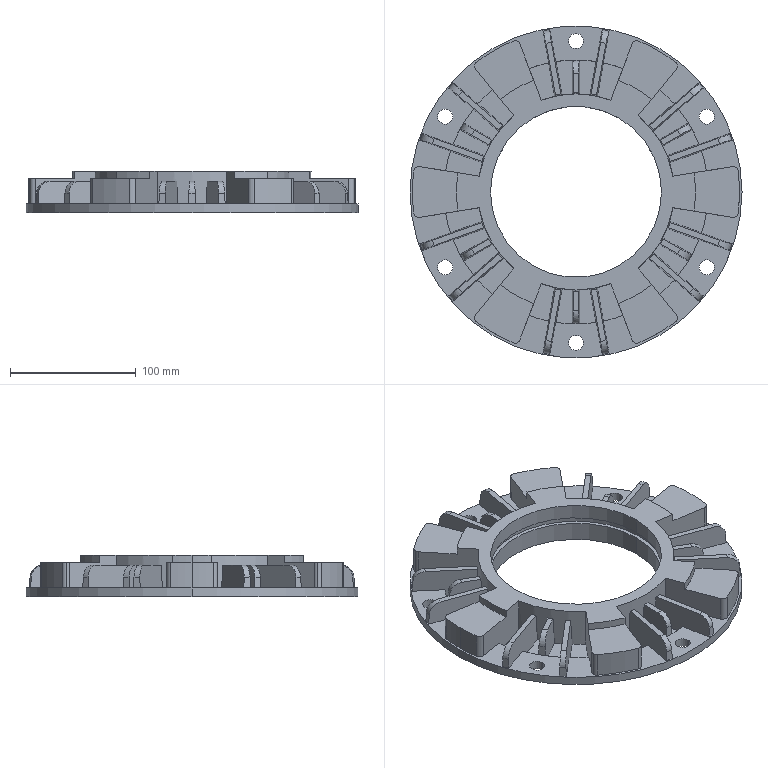Part | SolidWorks | features BaseBody 1 | 1 solid | 245 faces | box 264 x 264 x 33 mm | volume 629435 mm3 | plane 143 | cylinder 102 | commonest cylinder face diameters 12 x24 20 x18 210 x18 8 x14 190 x7 260 x7